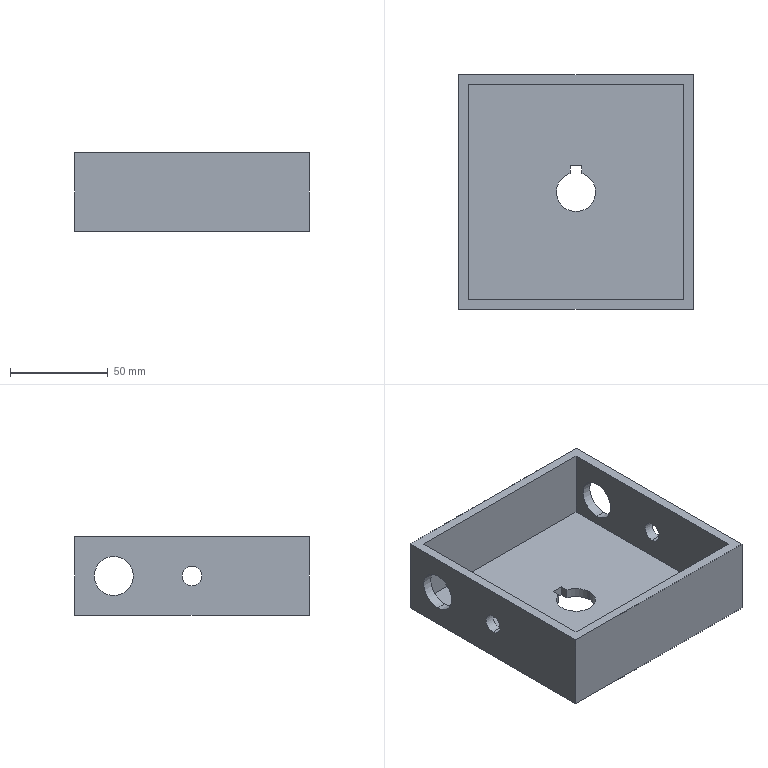Part | SolidWorks | features ICE 3, Extrusion 1 | 1 solid | 25 faces | box 120 x 120 x 40 mm | volume 146891 mm3 | plane 14 | cylinder 11 | commonest cylinder face diameters 20 x7 10 x4
STEP:
#1=CARTESIAN_POINT('',(10.,0.,5.));
#2=VERTEX_POINT('',#1);
#3=CARTESIAN_POINT('',(-10.,0.,5.));
#4=VERTEX_POINT('',#3);
#5=CARTESIAN_POINT('',(0.,0.,5.));
#6=DIRECTION('',(0.,0.,-1.));
#7=DIRECTION('',(-1.,0.,0.));
#8=AXIS2_PLACEMENT_3D('',#5,#6,#7);
#9=CIRCLE('',#8,10.);
#10=EDGE_CURVE('',#2,#4,#9,.T.);
#11=ORIENTED_EDGE('',*,*,#10,.F.);
#12=CARTESIAN_POINT('',(10.,0.,0.));
#13=VERTEX_POINT('',#12);
#14=CARTESIAN_POINT('',(10.,0.,40.));
#15=DIRECTION('',(0.,0.,-1.));
#16=VECTOR('',#15,1000.);
#17=LINE('',#14,#16);
#18=EDGE_CURVE('',#2,#13,#17,.T.);
#19=ORIENTED_EDGE('',*,*,#18,.T.);
#20=CARTESIAN_POINT('',(-10.,0.,0.));
#21=VERTEX_POINT('',#20);
#22=CARTESIAN_POINT('',(0.,0.,0.));
#23=DIRECTION('',(0.,0.,-1.));
#24=DIRECTION('',(-1.,0.,0.));
#25=AXIS2_PLACEMENT_3D('',#22,#23,#24);
#26=CIRCLE('',#25,10.);
#27=EDGE_CURVE('',#13,#21,#26,.T.);
#28=ORIENTED_EDGE('',*,*,#27,.T.);
#29=CARTESIAN_POINT('',(-10.,0.,40.));
#30=DIRECTION('',(0.,0.,-1.));
#31=VECTOR('',#30,1000.);
#32=LINE('',#29,#31);
#33=EDGE_CURVE('',#4,#21,#32,.T.);
#34=ORIENTED_EDGE('',*,*,#33,.F.);
#35=EDGE_LOOP('',(#11,#19,#28,#34));
#36=FACE_OUTER_BOUND('',#35,.T.);
#37=CARTESIAN_POINT('',(0.,0.,40.));
#38=DIRECTION('',(0.,0.,-1.));
#39=DIRECTION('',(-1.,0.,0.));
#40=AXIS2_PLACEMENT_3D('',#37,#38,#39);
#41=CYLINDRICAL_SURFACE('',#40,10.);
#42=ADVANCED_FACE('',(#36),#41,.F.);
#43=CARTESIAN_POINT('',(-3.,9.539,5.));
#44=VERTEX_POINT('',#43);
#45=CARTESIAN_POINT('',(0.,0.,5.));
#46=DIRECTION('',(0.,0.,-1.));
#47=DIRECTION('',(-1.,0.,0.));
#48=AXIS2_PLACEMENT_3D('',#45,#46,#47);
#49=CIRCLE('',#48,10.);
#50=EDGE_CURVE('',#4,#44,#49,.T.);
#51=ORIENTED_EDGE('',*,*,#50,.F.);
#52=ORIENTED_EDGE('',*,*,#33,.T.);
#53=CARTESIAN_POINT('',(-3.,9.539,0.));
#54=VERTEX_POINT('',#53);
#55=CARTESIAN_POINT('',(0.,0.,0.));
#56=DIRECTION('',(0.,0.,-1.));
#57=DIRECTION('',(-1.,0.,0.));
#58=AXIS2_PLACEMENT_3D('',#55,#56,#57);
#59=CIRCLE('',#58,10.);
#60=EDGE_CURVE('',#21,#54,#59,.T.);
#61=ORIENTED_EDGE('',*,*,#60,.T.);
#62=CARTESIAN_POINT('',(-3.,9.539,40.));
#63=DIRECTION('',(0.,0.,-1.));
#64=VECTOR('',#63,1000.);
#65=LINE('',#62,#64);
#66=EDGE_CURVE('',#44,#54,#65,.T.);
#67=ORIENTED_EDGE('',*,*,#66,.F.);
#68=EDGE_LOOP('',(#51,#52,#61,#67));
#69=FACE_OUTER_BOUND('',#68,.T.);
#70=CARTESIAN_POINT('',(0.,0.,40.));
#71=DIRECTION('',(0.,0.,-1.));
#72=DIRECTION('',(-1.,0.,0.));
#73=AXIS2_PLACEMENT_3D('',#70,#71,#72);
#74=CYLINDRICAL_SURFACE('',#73,10.);
#75=ADVANCED_FACE('',(#69),#74,.F.);
#76=CARTESIAN_POINT('',(-60.,40.,30.));
#77=VERTEX_POINT('',#76);
#78=CARTESIAN_POINT('',(-60.,40.,10.));
#79=VERTEX_POINT('',#78);
#80=CARTESIAN_POINT('',(-60.,40.,20.));
#81=DIRECTION('',(1.,0.,0.));
#82=DIRECTION('',(0.,0.,-1.));
#83=AXIS2_PLACEMENT_3D('',#80,#81,#82);
#84=CIRCLE('',#83,10.);
#85=EDGE_CURVE('',#77,#79,#84,.T.);
#86=ORIENTED_EDGE('',*,*,#85,.F.);
#87=CARTESIAN_POINT('',(-55.,40.,30.));
#88=VERTEX_POINT('',#87);
#89=CARTESIAN_POINT('',(-60.,40.,30.));
#90=DIRECTION('',(1.,0.,0.));
#91=VECTOR('',#90,1000.);
#92=LINE('',#89,#91);
#93=EDGE_CURVE('',#77,#88,#92,.T.);
#94=ORIENTED_EDGE('',*,*,#93,.T.);
#95=CARTESIAN_POINT('',(-55.,40.,10.));
#96=VERTEX_POINT('',#95);
#97=CARTESIAN_POINT('',(-55.,40.,20.));
#98=DIRECTION('',(1.,0.,0.));
#99=DIRECTION('',(0.,0.,1.));
#100=AXIS2_PLACEMENT_3D('',#97,#98,#99);
#101=CIRCLE('',#100,10.);
#102=EDGE_CURVE('',#88,#96,#101,.T.);
#103=ORIENTED_EDGE('',*,*,#102,.T.);
#104=CARTESIAN_POINT('',(-60.,40.,10.));
#105=DIRECTION('',(1.,0.,0.));
#106=VECTOR('',#105,1000.);
#107=LINE('',#104,#106);
#108=EDGE_CURVE('',#79,#96,#107,.T.);
#109=ORIENTED_EDGE('',*,*,#108,.F.);
#110=EDGE_LOOP('',(#86,#94,#103,#109));
#111=FACE_OUTER_BOUND('',#110,.T.);
#112=CARTESIAN_POINT('',(-60.,40.,20.));
#113=DIRECTION('',(1.,0.,0.));
#114=DIRECTION('',(0.,0.,-1.));
#115=AXIS2_PLACEMENT_3D('',#112,#113,#114);
#116=CYLINDRICAL_SURFACE('',#115,10.);
#117=ADVANCED_FACE('',(#111),#116,.F.);
#118=CARTESIAN_POINT('',(-60.,0.,25.));
#119=VERTEX_POINT('',#118);
#120=CARTESIAN_POINT('',(-60.,0.,15.));
#121=VERTEX_POINT('',#120);
#122=CARTESIAN_POINT('',(-60.,0.,20.));
#123=DIRECTION('',(1.,0.,0.));
#124=DIRECTION('',(0.,0.,-1.));
#125=AXIS2_PLACEMENT_3D('',#122,#123,#124);
#126=CIRCLE('',#125,5.);
#127=EDGE_CURVE('',#119,#121,#126,.T.);
#128=ORIENTED_EDGE('',*,*,#127,.F.);
#129=CARTESIAN_POINT('',(-55.,0.,25.));
#130=VERTEX_POINT('',#129);
#131=CARTESIAN_POINT('',(-60.,0.,25.));
#132=DIRECTION('',(1.,0.,0.));
#133=VECTOR('',#132,1000.);
#134=LINE('',#131,#133);
#135=EDGE_CURVE('',#119,#130,#134,.T.);
#136=ORIENTED_EDGE('',*,*,#135,.T.);
#137=CARTESIAN_POINT('',(-55.,0.,15.));
#138=VERTEX_POINT('',#137);
#139=CARTESIAN_POINT('',(-55.,0.,20.));
#140=DIRECTION('',(1.,0.,0.));
#141=DIRECTION('',(0.,0.,1.));
#142=AXIS2_PLACEMENT_3D('',#139,#140,#141);
#143=CIRCLE('',#142,5.);
#144=EDGE_CURVE('',#130,#138,#143,.T.);
#145=ORIENTED_EDGE('',*,*,#144,.T.);
#146=CARTESIAN_POINT('',(-60.,0.,15.));
#147=DIRECTION('',(1.,0.,0.));
#148=VECTOR('',#147,1000.);
#149=LINE('',#146,#148);
#150=EDGE_CURVE('',#121,#138,#149,.T.);
#151=ORIENTED_EDGE('',*,*,#150,.F.);
#152=EDGE_LOOP('',(#128,#136,#145,#151));
#153=FACE_OUTER_BOUND('',#152,.T.);
#154=CARTESIAN_POINT('',(-60.,0.,20.));
#155=DIRECTION('',(1.,0.,0.));
#156=DIRECTION('',(0.,0.,-1.));
#157=AXIS2_PLACEMENT_3D('',#154,#155,#156);
#158=CYLINDRICAL_SURFACE('',#157,5.);
#159=ADVANCED_FACE('',(#153),#158,.F.);
#160=CARTESIAN_POINT('',(55.,40.,10.));
#161=VERTEX_POINT('',#160);
#162=CARTESIAN_POINT('',(55.,40.,30.));
#163=VERTEX_POINT('',#162);
#164=CARTESIAN_POINT('',(55.,40.,20.));
#165=DIRECTION('',(-1.,0.,0.));
#166=DIRECTION('',(0.,0.,-1.));
#167=AXIS2_PLACEMENT_3D('',#164,#165,#166);
#168=CIRCLE('',#167,10.);
#169=EDGE_CURVE('',#161,#163,#168,.T.);
#170=ORIENTED_EDGE('',*,*,#169,.T.);
#171=CARTESIAN_POINT('',(60.,40.,30.));
#172=VERTEX_POINT('',#171);
#173=CARTESIAN_POINT('',(-60.,40.,30.));
#174=DIRECTION('',(1.,0.,0.));
#175=VECTOR('',#174,1000.);
#176=LINE('',#173,#175);
#177=EDGE_CURVE('',#163,#172,#176,.T.);
#178=ORIENTED_EDGE('',*,*,#177,.T.);
#179=CARTESIAN_POINT('',(60.,40.,10.));
#180=VERTEX_POINT('',#179);
#181=CARTESIAN_POINT('',(60.,40.,20.));
#182=DIRECTION('',(1.,0.,0.));
#183=DIRECTION('',(0.,0.,-1.));
#184=AXIS2_PLACEMENT_3D('',#181,#182,#183);
#185=CIRCLE('',#184,10.);
#186=EDGE_CURVE('',#172,#180,#185,.T.);
#187=ORIENTED_EDGE('',*,*,#186,.T.);
#188=CARTESIAN_POINT('',(-60.,40.,10.));
#189=DIRECTION('',(1.,0.,0.));
#190=VECTOR('',#189,1000.);
#191=LINE('',#188,#190);
#192=EDGE_CURVE('',#161,#180,#191,.T.);
#193=ORIENTED_EDGE('',*,*,#192,.F.);
#194=EDGE_LOOP('',(#170,#178,#187,#193));
#195=FACE_OUTER_BOUND('',#194,.T.);
#196=CARTESIAN_POINT('',(-60.,40.,20.));
#197=DIRECTION('',(1.,0.,0.));
#198=DIRECTION('',(0.,0.,-1.));
#199=AXIS2_PLACEMENT_3D('',#196,#197,#198);
#200=CYLINDRICAL_SURFACE('',#199,10.);
#201=ADVANCED_FACE('',(#195),#200,.F.);
#202=CARTESIAN_POINT('',(55.,0.,15.));
#203=VERTEX_POINT('',#202);
#204=CARTESIAN_POINT('',(55.,0.,25.));
#205=VERTEX_POINT('',#204);
#206=CARTESIAN_POINT('',(55.,0.,20.));
#207=DIRECTION('',(-1.,0.,0.));
#208=DIRECTION('',(0.,0.,-1.));
#209=AXIS2_PLACEMENT_3D('',#206,#207,#208);
#210=CIRCLE('',#209,5.);
#211=EDGE_CURVE('',#203,#205,#210,.T.);
#212=ORIENTED_EDGE('',*,*,#211,.T.);
#213=CARTESIAN_POINT('',(60.,0.,25.));
#214=VERTEX_POINT('',#213);
#215=CARTESIAN_POINT('',(-60.,0.,25.));
#216=DIRECTION('',(1.,0.,0.));
#217=VECTOR('',#216,1000.);
#218=LINE('',#215,#217);
#219=EDGE_CURVE('',#205,#214,#218,.T.);
#220=ORIENTED_EDGE('',*,*,#219,.T.);
#221=CARTESIAN_POINT('',(60.,0.,15.));
#222=VERTEX_POINT('',#221);
#223=CARTESIAN_POINT('',(60.,0.,20.));
#224=DIRECTION('',(1.,0.,0.));
#225=DIRECTION('',(0.,0.,-1.));
#226=AXIS2_PLACEMENT_3D('',#223,#224,#225);
#227=CIRCLE('',#226,5.);
#228=EDGE_CURVE('',#214,#222,#227,.T.);
#229=ORIENTED_EDGE('',*,*,#228,.T.);
#230=CARTESIAN_POINT('',(-60.,0.,15.));
#231=DIRECTION('',(1.,0.,0.));
#232=VECTOR('',#231,1000.);
#233=LINE('',#230,#232);
#234=EDGE_CURVE('',#203,#222,#233,.T.);
#235=ORIENTED_EDGE('',*,*,#234,.F.);
#236=EDGE_LOOP('',(#212,#220,#229,#235));
#237=FACE_OUTER_BOUND('',#236,.T.);
#238=CARTESIAN_POINT('',(-60.,0.,20.));
#239=DIRECTION('',(1.,0.,0.));
#240=DIRECTION('',(0.,0.,-1.));
#241=AXIS2_PLACEMENT_3D('',#238,#239,#240);
#242=CYLINDRICAL_SURFACE('',#241,5.);
#243=ADVANCED_FACE('',(#237),#242,.F.);
#244=ORIENTED_EDGE('',*,*,#219,.F.);
#245=CARTESIAN_POINT('',(55.,0.,20.));
#246=DIRECTION('',(-1.,0.,0.));
#247=DIRECTION('',(0.,0.,-1.));
#248=AXIS2_PLACEMENT_3D('',#245,#246,#247);
#249=CIRCLE('',#248,5.);
#250=EDGE_CURVE('',#205,#203,#249,.T.);
#251=ORIENTED_EDGE('',*,*,#250,.T.);
#252=ORIENTED_EDGE('',*,*,#234,.T.);
#253=CARTESIAN_POINT('',(60.,0.,20.));
#254=DIRECTION('',(1.,0.,0.));
#255=DIRECTION('',(0.,0.,-1.));
#256=AXIS2_PLACEMENT_3D('',#253,#254,#255);
#257=CIRCLE('',#256,5.);
#258=EDGE_CURVE('',#222,#214,#257,.T.);
#259=ORIENTED_EDGE('',*,*,#258,.T.);
#260=EDGE_LOOP('',(#244,#251,#252,#259));
#261=FACE_OUTER_BOUND('',#260,.T.);
#262=CARTESIAN_POINT('',(-60.,0.,20.));
#263=DIRECTION('',(1.,0.,0.));
#264=DIRECTION('',(0.,0.,-1.));
#265=AXIS2_PLACEMENT_3D('',#262,#263,#264);
#266=CYLINDRICAL_SURFACE('',#265,5.);
#267=ADVANCED_FACE('',(#261),#266,.F.);
#268=ORIENTED_EDGE('',*,*,#177,.F.);
#269=CARTESIAN_POINT('',(55.,40.,20.));
#270=DIRECTION('',(-1.,0.,0.));
#271=DIRECTION('',(0.,0.,-1.));
#272=AXIS2_PLACEMENT_3D('',#269,#270,#271);
#273=CIRCLE('',#272,10.);
#274=EDGE_CURVE('',#163,#161,#273,.T.);
#275=ORIENTED_EDGE('',*,*,#274,.T.);
#276=ORIENTED_EDGE('',*,*,#192,.T.);
#277=CARTESIAN_POINT('',(60.,40.,20.));
#278=DIRECTION('',(1.,0.,0.));
#279=DIRECTION('',(0.,0.,-1.));
#280=AXIS2_PLACEMENT_3D('',#277,#278,#279);
#281=CIRCLE('',#280,10.);
#282=EDGE_CURVE('',#180,#172,#281,.T.);
#283=ORIENTED_EDGE('',*,*,#282,.T.);
#284=EDGE_LOOP('',(#268,#275,#276,#283));
#285=FACE_OUTER_BOUND('',#284,.T.);
#286=CARTESIAN_POINT('',(-60.,40.,20.));
#287=DIRECTION('',(1.,0.,0.));
#288=DIRECTION('',(0.,0.,-1.));
#289=AXIS2_PLACEMENT_3D('',#286,#287,#288);
#290=CYLINDRICAL_SURFACE('',#289,10.);
#291=ADVANCED_FACE('',(#285),#290,.F.);
#292=ORIENTED_EDGE('',*,*,#282,.F.);
#293=ORIENTED_EDGE('',*,*,#186,.F.);
#294=EDGE_LOOP('',(#292,#293));
#295=FACE_BOUND('',#294,.T.);
#296=ORIENTED_EDGE('',*,*,#258,.F.);
#297=ORIENTED_EDGE('',*,*,#228,.F.);
#298=EDGE_LOOP('',(#296,#297));
#299=FACE_BOUND('',#298,.T.);
#300=CARTESIAN_POINT('',(60.,-60.,0.));
#301=VERTEX_POINT('',#300);
#302=CARTESIAN_POINT('',(60.,60.,0.));
#303=VERTEX_POINT('',#302);
#304=CARTESIAN_POINT('',(60.,-60.,0.));
#305=DIRECTION('',(0.,1.,0.));
#306=VECTOR('',#305,1000.);
#307=LINE('',#304,#306);
#308=EDGE_CURVE('',#301,#303,#307,.T.);
#309=ORIENTED_EDGE('',*,*,#308,.T.);
#310=CARTESIAN_POINT('',(60.,60.,40.));
#311=VERTEX_POINT('',#310);
#312=CARTESIAN_POINT('',(60.,60.,40.));
#313=DIRECTION('',(0.,0.,-1.));
#314=VECTOR('',#313,1000.);
#315=LINE('',#312,#314);
#316=EDGE_CURVE('',#311,#303,#315,.T.);
#317=ORIENTED_EDGE('',*,*,#316,.F.);
#318=CARTESIAN_POINT('',(60.,-60.,40.));
#319=VERTEX_POINT('',#318);
#320=CARTESIAN_POINT('',(60.,-60.,40.));
#321=DIRECTION('',(0.,1.,0.));
#322=VECTOR('',#321,1000.);
#323=LINE('',#320,#322);
#324=EDGE_CURVE('',#319,#311,#323,.T.);
#325=ORIENTED_EDGE('',*,*,#324,.F.);
#326=CARTESIAN_POINT('',(60.,-60.,40.));
#327=DIRECTION('',(0.,0.,-1.));
#328=VECTOR('',#327,1000.);
#329=LINE('',#326,#328);
#330=EDGE_CURVE('',#319,#301,#329,.T.);
#331=ORIENTED_EDGE('',*,*,#330,.T.);
#332=EDGE_LOOP('',(#309,#317,#325,#331));
#333=FACE_OUTER_BOUND('',#332,.T.);
#334=CARTESIAN_POINT('',(60.,-60.,40.));
#335=DIRECTION('',(-1.,0.,0.));
#336=DIRECTION('',(0.,0.,1.));
#337=AXIS2_PLACEMENT_3D('',#334,#335,#336);
#338=PLANE('',#337);
#339=ADVANCED_FACE('',(#295,#299,#333),#338,.F.);
#340=CARTESIAN_POINT('',(-60.,60.,0.));
#341=VERTEX_POINT('',#340);
#342=CARTESIAN_POINT('',(-60.,60.,0.));
#343=DIRECTION('',(-1.,0.,0.));
#344=VECTOR('',#343,1000.);
#345=LINE('',#342,#344);
#346=EDGE_CURVE('',#303,#341,#345,.T.);
#347=ORIENTED_EDGE('',*,*,#346,.T.);
#348=CARTESIAN_POINT('',(-60.,60.,40.));
#349=VERTEX_POINT('',#348);
#350=CARTESIAN_POINT('',(-60.,60.,40.));
#351=DIRECTION('',(0.,0.,-1.));
#352=VECTOR('',#351,1000.);
#353=LINE('',#350,#352);
#354=EDGE_CURVE('',#349,#341,#353,.T.);
#355=ORIENTED_EDGE('',*,*,#354,.F.);
#356=CARTESIAN_POINT('',(-60.,60.,40.));
#357=DIRECTION('',(-1.,0.,0.));
#358=VECTOR('',#357,1000.);
#359=LINE('',#356,#358);
#360=EDGE_CURVE('',#311,#349,#359,.T.);
#361=ORIENTED_EDGE('',*,*,#360,.F.);
#362=ORIENTED_EDGE('',*,*,#316,.T.);
#363=EDGE_LOOP('',(#347,#355,#361,#362));
#364=FACE_OUTER_BOUND('',#363,.T.);
#365=CARTESIAN_POINT('',(-60.,60.,40.));
#366=DIRECTION('',(0.,-1.,0.));
#367=DIRECTION('',(0.,0.,-1.));
#368=AXIS2_PLACEMENT_3D('',#365,#366,#367);
#369=PLANE('',#368);
#370=ADVANCED_FACE('',(#364),#369,.F.);
#371=CARTESIAN_POINT('',(-60.,40.,20.));
#372=DIRECTION('',(1.,0.,0.));
#373=DIRECTION('',(0.,0.,-1.));
#374=AXIS2_PLACEMENT_3D('',#371,#372,#373);
#375=CIRCLE('',#374,10.);
#376=EDGE_CURVE('',#79,#77,#375,.T.);
#377=ORIENTED_EDGE('',*,*,#376,.T.);
#378=ORIENTED_EDGE('',*,*,#85,.T.);
#379=EDGE_LOOP('',(#377,#378));
#380=FACE_BOUND('',#379,.T.);
#381=CARTESIAN_POINT('',(-60.,0.,20.));
#382=DIRECTION('',(1.,0.,0.));
#383=DIRECTION('',(0.,0.,-1.));
#384=AXIS2_PLACEMENT_3D('',#381,#382,#383);
#385=CIRCLE('',#384,5.);
#386=EDGE_CURVE('',#121,#119,#385,.T.);
#387=ORIENTED_EDGE('',*,*,#386,.T.);
#388=ORIENTED_EDGE('',*,*,#127,.T.);
#389=EDGE_LOOP('',(#387,#388));
#390=FACE_BOUND('',#389,.T.);
#391=CARTESIAN_POINT('',(-60.,-60.,0.));
#392=VERTEX_POINT('',#391);
#393=CARTESIAN_POINT('',(-60.,-60.,0.));
#394=DIRECTION('',(0.,-1.,0.));
#395=VECTOR('',#394,1000.);
#396=LINE('',#393,#395);
#397=EDGE_CURVE('',#341,#392,#396,.T.);
#398=ORIENTED_EDGE('',*,*,#397,.T.);
#399=CARTESIAN_POINT('',(-60.,-60.,40.));
#400=VERTEX_POINT('',#399);
#401=CARTESIAN_POINT('',(-60.,-60.,40.));
#402=DIRECTION('',(0.,0.,-1.));
#403=VECTOR('',#402,1000.);
#404=LINE('',#401,#403);
#405=EDGE_CURVE('',#400,#392,#404,.T.);
#406=ORIENTED_EDGE('',*,*,#405,.F.);
#407=CARTESIAN_POINT('',(-60.,-60.,40.));
#408=DIRECTION('',(0.,-1.,0.));
#409=VECTOR('',#408,1000.);
#410=LINE('',#407,#409);
#411=EDGE_CURVE('',#349,#400,#410,.T.);
#412=ORIENTED_EDGE('',*,*,#411,.F.);
#413=ORIENTED_EDGE('',*,*,#354,.T.);
#414=EDGE_LOOP('',(#398,#406,#412,#413));
#415=FACE_OUTER_BOUND('',#414,.T.);
#416=CARTESIAN_POINT('',(-60.,-60.,40.));
#417=DIRECTION('',(1.,0.,0.));
#418=DIRECTION('',(0.,0.,-1.));
#419=AXIS2_PLACEMENT_3D('',#416,#417,#418);
#420=PLANE('',#419);
#421=ADVANCED_FACE('',(#380,#390,#415),#420,.F.);
#422=CARTESIAN_POINT('',(-60.,-60.,0.));
#423=DIRECTION('',(1.,0.,0.));
#424=VECTOR('',#423,1000.);
#425=LINE('',#422,#424);
#426=EDGE_CURVE('',#392,#301,#425,.T.);
#427=ORIENTED_EDGE('',*,*,#426,.T.);
#428=ORIENTED_EDGE('',*,*,#330,.F.);
#429=CARTESIAN_POINT('',(-60.,-60.,40.));
#430=DIRECTION('',(1.,0.,0.));
#431=VECTOR('',#430,1000.);
#432=LINE('',#429,#431);
#433=EDGE_CURVE('',#400,#319,#432,.T.);
#434=ORIENTED_EDGE('',*,*,#433,.F.);
#435=ORIENTED_EDGE('',*,*,#405,.T.);
#436=EDGE_LOOP('',(#427,#428,#434,#435));
#437=FACE_OUTER_BOUND('',#436,.T.);
#438=CARTESIAN_POINT('',(-60.,-60.,40.));
#439=DIRECTION('',(0.,1.,0.));
#440=DIRECTION('',(0.,0.,1.));
#441=AXIS2_PLACEMENT_3D('',#438,#439,#440);
#442=PLANE('',#441);
#443=ADVANCED_FACE('',(#437),#442,.F.);
#444=CARTESIAN_POINT('',(55.,55.,40.));
#445=VERTEX_POINT('',#444);
#446=CARTESIAN_POINT('',(-55.,55.,40.));
#447=VERTEX_POINT('',#446);
#448=CARTESIAN_POINT('',(-55.,55.,40.));
#449=DIRECTION('',(-1.,0.,0.));
#450=VECTOR('',#449,1000.);
#451=LINE('',#448,#450);
#452=EDGE_CURVE('',#445,#447,#451,.T.);
#453=ORIENTED_EDGE('',*,*,#452,.F.);
#454=CARTESIAN_POINT('',(55.,-55.,40.));
#455=VERTEX_POINT('',#454);
#456=CARTESIAN_POINT('',(55.,-55.,40.));
#457=DIRECTION('',(0.,1.,0.));
#458=VECTOR('',#457,1000.);
#459=LINE('',#456,#458);
#460=EDGE_CURVE('',#455,#445,#459,.T.);
#461=ORIENTED_EDGE('',*,*,#460,.F.);
#462=CARTESIAN_POINT('',(-55.,-55.,40.));
#463=VERTEX_POINT('',#462);
#464=CARTESIAN_POINT('',(-55.,-55.,40.));
#465=DIRECTION('',(1.,0.,0.));
#466=VECTOR('',#465,1000.);
#467=LINE('',#464,#466);
#468=EDGE_CURVE('',#463,#455,#467,.T.);
#469=ORIENTED_EDGE('',*,*,#468,.F.);
#470=CARTESIAN_POINT('',(-55.,-55.,40.));
#471=DIRECTION('',(0.,-1.,0.));
#472=VECTOR('',#471,1000.);
#473=LINE('',#470,#472);
#474=EDGE_CURVE('',#447,#463,#473,.T.);
#475=ORIENTED_EDGE('',*,*,#474,.F.);
#476=EDGE_LOOP('',(#453,#461,#469,#475));
#477=FACE_BOUND('',#476,.T.);
#478=ORIENTED_EDGE('',*,*,#324,.T.);
#479=ORIENTED_EDGE('',*,*,#360,.T.);
#480=ORIENTED_EDGE('',*,*,#411,.T.);
#481=ORIENTED_EDGE('',*,*,#433,.T.);
#482=EDGE_LOOP('',(#478,#479,#480,#481));
#483=FACE_OUTER_BOUND('',#482,.T.);
#484=CARTESIAN_POINT('',(0.,0.,40.));
#485=DIRECTION('',(0.,0.,-1.));
#486=DIRECTION('',(-1.,0.,0.));
#487=AXIS2_PLACEMENT_3D('',#484,#485,#486);
#488=PLANE('',#487);
#489=ADVANCED_FACE('',(#477,#483),#488,.F.);
#490=CARTESIAN_POINT('',(3.,9.539,0.));
#491=VERTEX_POINT('',#490);
#492=CARTESIAN_POINT('',(0.,0.,0.));
#493=DIRECTION('',(0.,0.,-1.));
#494=DIRECTION('',(-1.,0.,0.));
#495=AXIS2_PLACEMENT_3D('',#492,#493,#494);
#496=CIRCLE('',#495,10.);
#497=EDGE_CURVE('',#491,#13,#496,.T.);
#498=ORIENTED_EDGE('',*,*,#497,.F.);
#499=CARTESIAN_POINT('',(3.,13.539,0.));
#500=VERTEX_POINT('',#499);
#501=CARTESIAN_POINT('',(3.,9.539,0.));
#502=DIRECTION('',(0.,-1.,0.));
#503=VECTOR('',#502,1000.);
#504=LINE('',#501,#503);
#505=EDGE_CURVE('',#500,#491,#504,.T.);
#506=ORIENTED_EDGE('',*,*,#505,.F.);
#507=CARTESIAN_POINT('',(-3.,13.539,0.));
#508=VERTEX_POINT('',#507);
#509=CARTESIAN_POINT('',(-3.,13.539,0.));
#510=DIRECTION('',(1.,0.,0.));
#511=VECTOR('',#510,1000.);
#512=LINE('',#509,#511);
#513=EDGE_CURVE('',#508,#500,#512,.T.);
#514=ORIENTED_EDGE('',*,*,#513,.F.);
#515=CARTESIAN_POINT('',(-3.,9.539,0.));
#516=DIRECTION('',(0.,1.,0.));
#517=VECTOR('',#516,1000.);
#518=LINE('',#515,#517);
#519=EDGE_CURVE('',#54,#508,#518,.T.);
#520=ORIENTED_EDGE('',*,*,#519,.F.);
#521=ORIENTED_EDGE('',*,*,#60,.F.);
#522=ORIENTED_EDGE('',*,*,#27,.F.);
#523=EDGE_LOOP('',(#498,#506,#514,#520,#521,#522));
#524=FACE_BOUND('',#523,.T.);
#525=ORIENTED_EDGE('',*,*,#308,.F.);
#526=ORIENTED_EDGE('',*,*,#426,.F.);
#527=ORIENTED_EDGE('',*,*,#397,.F.);
#528=ORIENTED_EDGE('',*,*,#346,.F.);
#529=EDGE_LOOP('',(#525,#526,#527,#528));
#530=FACE_OUTER_BOUND('',#529,.T.);
#531=CARTESIAN_POINT('',(0.,0.,0.));
#532=DIRECTION('',(0.,0.,-1.));
#533=DIRECTION('',(-1.,0.,0.));
#534=AXIS2_PLACEMENT_3D('',#531,#532,#533);
#535=PLANE('',#534);
#536=ADVANCED_FACE('',(#524,#530),#535,.T.);
#537=ORIENTED_EDGE('',*,*,#135,.F.);
#538=ORIENTED_EDGE('',*,*,#386,.F.);
#539=ORIENTED_EDGE('',*,*,#150,.T.);
#540=CARTESIAN_POINT('',(-55.,0.,20.));
#541=DIRECTION('',(1.,0.,0.));
#542=DIRECTION('',(0.,0.,1.));
#543=AXIS2_PLACEMENT_3D('',#540,#541,#542);
#544=CIRCLE('',#543,5.);
#545=EDGE_CURVE('',#138,#130,#544,.T.);
#546=ORIENTED_EDGE('',*,*,#545,.T.);
#547=EDGE_LOOP('',(#537,#538,#539,#546));
#548=FACE_OUTER_BOUND('',#547,.T.);
#549=CARTESIAN_POINT('',(-60.,0.,20.));
#550=DIRECTION('',(1.,0.,0.));
#551=DIRECTION('',(0.,0.,-1.));
#552=AXIS2_PLACEMENT_3D('',#549,#550,#551);
#553=CYLINDRICAL_SURFACE('',#552,5.);
#554=ADVANCED_FACE('',(#548),#553,.F.);
#555=ORIENTED_EDGE('',*,*,#93,.F.);
#556=ORIENTED_EDGE('',*,*,#376,.F.);
#557=ORIENTED_EDGE('',*,*,#108,.T.);
#558=CARTESIAN_POINT('',(-55.,40.,20.));
#559=DIRECTION('',(1.,0.,0.));
#560=DIRECTION('',(0.,0.,1.));
#561=AXIS2_PLACEMENT_3D('',#558,#559,#560);
#562=CIRCLE('',#561,10.);
#563=EDGE_CURVE('',#96,#88,#562,.T.);
#564=ORIENTED_EDGE('',*,*,#563,.T.);
#565=EDGE_LOOP('',(#555,#556,#557,#564));
#566=FACE_OUTER_BOUND('',#565,.T.);
#567=CARTESIAN_POINT('',(-60.,40.,20.));
#568=DIRECTION('',(1.,0.,0.));
#569=DIRECTION('',(0.,0.,-1.));
#570=AXIS2_PLACEMENT_3D('',#567,#568,#569);
#571=CYLINDRICAL_SURFACE('',#570,10.);
#572=ADVANCED_FACE('',(#566),#571,.F.);
#573=ORIENTED_EDGE('',*,*,#169,.F.);
#574=ORIENTED_EDGE('',*,*,#274,.F.);
#575=EDGE_LOOP('',(#573,#574));
#576=FACE_BOUND('',#575,.T.);
#577=ORIENTED_EDGE('',*,*,#460,.T.);
#578=CARTESIAN_POINT('',(55.,55.,5.));
#579=VERTEX_POINT('',#578);
#580=CARTESIAN_POINT('',(55.,55.,5.));
#581=DIRECTION('',(0.,0.,1.));
#582=VECTOR('',#581,1000.);
#583=LINE('',#580,#582);
#584=EDGE_CURVE('',#579,#445,#583,.T.);
#585=ORIENTED_EDGE('',*,*,#584,.F.);
#586=CARTESIAN_POINT('',(55.,-55.,5.));
#587=VERTEX_POINT('',#586);
#588=CARTESIAN_POINT('',(55.,-55.,5.));
#589=DIRECTION('',(0.,1.,0.));
#590=VECTOR('',#589,1000.);
#591=LINE('',#588,#590);
#592=EDGE_CURVE('',#587,#579,#591,.T.);
#593=ORIENTED_EDGE('',*,*,#592,.F.);
#594=CARTESIAN_POINT('',(55.,-55.,5.));
#595=DIRECTION('',(0.,0.,1.));
#596=VECTOR('',#595,1000.);
#597=LINE('',#594,#596);
#598=EDGE_CURVE('',#587,#455,#597,.T.);
#599=ORIENTED_EDGE('',*,*,#598,.T.);
#600=EDGE_LOOP('',(#577,#585,#593,#599));
#601=FACE_OUTER_BOUND('',#600,.T.);
#602=ORIENTED_EDGE('',*,*,#211,.F.);
#603=ORIENTED_EDGE('',*,*,#250,.F.);
#604=EDGE_LOOP('',(#602,#603));
#605=FACE_BOUND('',#604,.T.);
#606=CARTESIAN_POINT('',(55.,-55.,5.));
#607=DIRECTION('',(1.,0.,0.));
#608=DIRECTION('',(0.,0.,-1.));
#609=AXIS2_PLACEMENT_3D('',#606,#607,#608);
#610=PLANE('',#609);
#611=ADVANCED_FACE('',(#576,#601,#605),#610,.F.);
#612=ORIENTED_EDGE('',*,*,#563,.F.);
#613=ORIENTED_EDGE('',*,*,#102,.F.);
#614=EDGE_LOOP('',(#612,#613));
#615=FACE_BOUND('',#614,.T.);
#616=ORIENTED_EDGE('',*,*,#474,.T.);
#617=CARTESIAN_POINT('',(-55.,-55.,5.));
#618=VERTEX_POINT('',#617);
#619=CARTESIAN_POINT('',(-55.,-55.,5.));
#620=DIRECTION('',(0.,0.,1.));
#621=VECTOR('',#620,1000.);
#622=LINE('',#619,#621);
#623=EDGE_CURVE('',#618,#463,#622,.T.);
#624=ORIENTED_EDGE('',*,*,#623,.F.);
#625=CARTESIAN_POINT('',(-55.,55.,5.));
#626=VERTEX_POINT('',#625);
#627=CARTESIAN_POINT('',(-55.,-55.,5.));
#628=DIRECTION('',(0.,-1.,0.));
#629=VECTOR('',#628,1000.);
#630=LINE('',#627,#629);
#631=EDGE_CURVE('',#626,#618,#630,.T.);
#632=ORIENTED_EDGE('',*,*,#631,.F.);
#633=CARTESIAN_POINT('',(-55.,55.,5.));
#634=DIRECTION('',(0.,0.,1.));
#635=VECTOR('',#634,1000.);
#636=LINE('',#633,#635);
#637=EDGE_CURVE('',#626,#447,#636,.T.);
#638=ORIENTED_EDGE('',*,*,#637,.T.);
#639=EDGE_LOOP('',(#616,#624,#632,#638));
#640=FACE_OUTER_BOUND('',#639,.T.);
#641=ORIENTED_EDGE('',*,*,#545,.F.);
#642=ORIENTED_EDGE('',*,*,#144,.F.);
#643=EDGE_LOOP('',(#641,#642));
#644=FACE_BOUND('',#643,.T.);
#645=CARTESIAN_POINT('',(-55.,-55.,5.));
#646=DIRECTION('',(-1.,0.,0.));
#647=DIRECTION('',(0.,0.,1.));
#648=AXIS2_PLACEMENT_3D('',#645,#646,#647);
#649=PLANE('',#648);
#650=ADVANCED_FACE('',(#615,#640,#644),#649,.F.);
#651=ORIENTED_EDGE('',*,*,#468,.T.);
#652=ORIENTED_EDGE('',*,*,#598,.F.);
#653=CARTESIAN_POINT('',(-55.,-55.,5.));
#654=DIRECTION('',(1.,0.,0.));
#655=VECTOR('',#654,1000.);
#656=LINE('',#653,#655);
#657=EDGE_CURVE('',#618,#587,#656,.T.);
#658=ORIENTED_EDGE('',*,*,#657,.F.);
#659=ORIENTED_EDGE('',*,*,#623,.T.);
#660=EDGE_LOOP('',(#651,#652,#658,#659));
#661=FACE_OUTER_BOUND('',#660,.T.);
#662=CARTESIAN_POINT('',(-55.,-55.,5.));
#663=DIRECTION('',(0.,-1.,0.));
#664=DIRECTION('',(0.,0.,-1.));
#665=AXIS2_PLACEMENT_3D('',#662,#663,#664);
#666=PLANE('',#665);
#667=ADVANCED_FACE('',(#661),#666,.F.);
#668=ORIENTED_EDGE('',*,*,#452,.T.);
#669=ORIENTED_EDGE('',*,*,#637,.F.);
#670=CARTESIAN_POINT('',(-55.,55.,5.));
#671=DIRECTION('',(-1.,0.,0.));
#672=VECTOR('',#671,1000.);
#673=LINE('',#670,#672);
#674=EDGE_CURVE('',#579,#626,#673,.T.);
#675=ORIENTED_EDGE('',*,*,#674,.F.);
#676=ORIENTED_EDGE('',*,*,#584,.T.);
#677=EDGE_LOOP('',(#668,#669,#675,#676));
#678=FACE_OUTER_BOUND('',#677,.T.);
#679=CARTESIAN_POINT('',(-55.,55.,5.));
#680=DIRECTION('',(0.,1.,0.));
#681=DIRECTION('',(0.,0.,1.));
#682=AXIS2_PLACEMENT_3D('',#679,#680,#681);
#683=PLANE('',#682);
#684=ADVANCED_FACE('',(#678),#683,.F.);
#685=CARTESIAN_POINT('',(3.,13.539,5.));
#686=VERTEX_POINT('',#685);
#687=CARTESIAN_POINT('',(3.,9.539,5.));
#688=VERTEX_POINT('',#687);
#689=CARTESIAN_POINT('',(3.,0.,5.));
#690=DIRECTION('',(0.,-1.,0.));
#691=VECTOR('',#690,1000.);
#692=LINE('',#689,#691);
#693=EDGE_CURVE('',#686,#688,#692,.T.);
#694=ORIENTED_EDGE('',*,*,#693,.T.);
#695=CARTESIAN_POINT('',(0.,0.,5.));
#696=DIRECTION('',(0.,0.,-1.));
#697=DIRECTION('',(-1.,0.,0.));
#698=AXIS2_PLACEMENT_3D('',#695,#696,#697);
#699=CIRCLE('',#698,10.);
#700=EDGE_CURVE('',#688,#2,#699,.T.);
#701=ORIENTED_EDGE('',*,*,#700,.T.);
#702=ORIENTED_EDGE('',*,*,#10,.T.);
#703=ORIENTED_EDGE('',*,*,#50,.T.);
#704=CARTESIAN_POINT('',(-3.,13.539,5.));
#705=VERTEX_POINT('',#704);
#706=CARTESIAN_POINT('',(-3.,0.,5.));
#707=DIRECTION('',(0.,1.,0.));
#708=VECTOR('',#707,1000.);
#709=LINE('',#706,#708);
#710=EDGE_CURVE('',#44,#705,#709,.T.);
#711=ORIENTED_EDGE('',*,*,#710,.T.);
#712=CARTESIAN_POINT('',(0.,13.539,5.));
#713=DIRECTION('',(1.,0.,0.));
#714=VECTOR('',#713,1000.);
#715=LINE('',#712,#714);
#716=EDGE_CURVE('',#705,#686,#715,.T.);
#717=ORIENTED_EDGE('',*,*,#716,.T.);
#718=EDGE_LOOP('',(#694,#701,#702,#703,#711,#717));
#719=FACE_BOUND('',#718,.T.);
#720=ORIENTED_EDGE('',*,*,#592,.T.);
#721=ORIENTED_EDGE('',*,*,#674,.T.);
#722=ORIENTED_EDGE('',*,*,#631,.T.);
#723=ORIENTED_EDGE('',*,*,#657,.T.);
#724=EDGE_LOOP('',(#720,#721,#722,#723));
#725=FACE_OUTER_BOUND('',#724,.T.);
#726=CARTESIAN_POINT('',(0.,0.,5.));
#727=DIRECTION('',(0.,0.,-1.));
#728=DIRECTION('',(-1.,0.,0.));
#729=AXIS2_PLACEMENT_3D('',#726,#727,#728);
#730=PLANE('',#729);
#731=ADVANCED_FACE('',(#719,#725),#730,.F.);
#732=ORIENTED_EDGE('',*,*,#18,.F.);
#733=ORIENTED_EDGE('',*,*,#700,.F.);
#734=CARTESIAN_POINT('',(3.,9.539,40.));
#735=DIRECTION('',(0.,0.,-1.));
#736=VECTOR('',#735,1000.);
#737=LINE('',#734,#736);
#738=EDGE_CURVE('',#688,#491,#737,.T.);
#739=ORIENTED_EDGE('',*,*,#738,.T.);
#740=ORIENTED_EDGE('',*,*,#497,.T.);
#741=EDGE_LOOP('',(#732,#733,#739,#740));
#742=FACE_OUTER_BOUND('',#741,.T.);
#743=CARTESIAN_POINT('',(0.,0.,40.));
#744=DIRECTION('',(0.,0.,-1.));
#745=DIRECTION('',(-1.,0.,0.));
#746=AXIS2_PLACEMENT_3D('',#743,#744,#745);
#747=CYLINDRICAL_SURFACE('',#746,10.);
#748=ADVANCED_FACE('',(#742),#747,.F.);
#749=CARTESIAN_POINT('',(3.,13.539,40.));
#750=DIRECTION('',(0.,0.,-1.));
#751=VECTOR('',#750,1000.);
#752=LINE('',#749,#751);
#753=EDGE_CURVE('',#686,#500,#752,.T.);
#754=ORIENTED_EDGE('',*,*,#753,.T.);
#755=ORIENTED_EDGE('',*,*,#505,.T.);
#756=ORIENTED_EDGE('',*,*,#738,.F.);
#757=ORIENTED_EDGE('',*,*,#693,.F.);
#758=EDGE_LOOP('',(#754,#755,#756,#757));
#759=FACE_OUTER_BOUND('',#758,.T.);
#760=CARTESIAN_POINT('',(3.,9.539,40.));
#761=DIRECTION('',(1.,0.,0.));
#762=DIRECTION('',(0.,0.,-1.));
#763=AXIS2_PLACEMENT_3D('',#760,#761,#762);
#764=PLANE('',#763);
#765=ADVANCED_FACE('',(#759),#764,.F.);
#766=CARTESIAN_POINT('',(-3.,13.539,40.));
#767=DIRECTION('',(0.,0.,-1.));
#768=VECTOR('',#767,1000.);
#769=LINE('',#766,#768);
#770=EDGE_CURVE('',#705,#508,#769,.T.);
#771=ORIENTED_EDGE('',*,*,#770,.T.);
#772=ORIENTED_EDGE('',*,*,#513,.T.);
#773=ORIENTED_EDGE('',*,*,#753,.F.);
#774=ORIENTED_EDGE('',*,*,#716,.F.);
#775=EDGE_LOOP('',(#771,#772,#773,#774));
#776=FACE_OUTER_BOUND('',#775,.T.);
#777=CARTESIAN_POINT('',(-3.,13.539,40.));
#778=DIRECTION('',(0.,1.,0.));
#779=DIRECTION('',(0.,0.,1.));
#780=AXIS2_PLACEMENT_3D('',#777,#778,#779);
#781=PLANE('',#780);
#782=ADVANCED_FACE('',(#776),#781,.F.);
#783=ORIENTED_EDGE('',*,*,#66,.T.);
#784=ORIENTED_EDGE('',*,*,#519,.T.);
#785=ORIENTED_EDGE('',*,*,#770,.F.);
#786=ORIENTED_EDGE('',*,*,#710,.F.);
#787=EDGE_LOOP('',(#783,#784,#785,#786));
#788=FACE_OUTER_BOUND('',#787,.T.);
#789=CARTESIAN_POINT('',(-3.,9.539,40.));
#790=DIRECTION('',(-1.,0.,0.));
#791=DIRECTION('',(0.,0.,1.));
#792=AXIS2_PLACEMENT_3D('',#789,#790,#791);
#793=PLANE('',#792);
#794=ADVANCED_FACE('',(#788),#793,.F.);
#795=CLOSED_SHELL('',(#42,#75,#117,#159,#201,#243,#267,#291,#339,#370,#421,#443,#489,#536,#554,#572,#611,#650,#667,#684,#731,#748,#765,#782,#794));
#796=MANIFOLD_SOLID_BREP('',#795);
#797=CARTESIAN_POINT('',(0.,0.,0.));
#798=DIRECTION('',(0.,0.,1.));
#799=DIRECTION('',(1.,0.,0.));
#800=AXIS2_PLACEMENT_3D('',#797,#798,#799);
#801=(LENGTH_UNIT()NAMED_UNIT(*)SI_UNIT(.MILLI.,.METRE.));
#802=UNCERTAINTY_MEASURE_WITH_UNIT(LENGTH_MEASURE(0.00001),#801,'','');
#803=(NAMED_UNIT(*)PLANE_ANGLE_UNIT()SI_UNIT($,.RADIAN.));
#804=(NAMED_UNIT(*)SI_UNIT($,.STERADIAN.)SOLID_ANGLE_UNIT());
#805=(GEOMETRIC_REPRESENTATION_CONTEXT(3)GLOBAL_UNCERTAINTY_ASSIGNED_CONTEXT((#802))GLOBAL_UNIT_ASSIGNED_CONTEXT((#801,#803,#804))REPRESENTATION_CONTEXT('',''));
#806=ADVANCED_BREP_SHAPE_REPRESENTATION('',(#796,#800),#805);